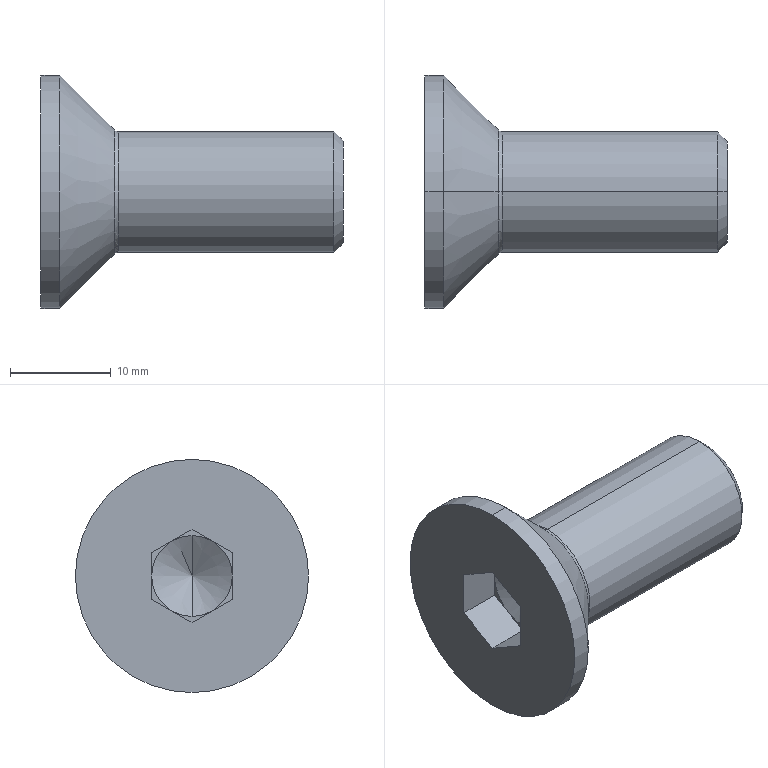Part | STEP file | 1 solid | 26 faces | box 30 x 23.12 x 23.12 mm | volume 4440 mm3 | plane 14 | cone 6 | cylinder 4 | torus 2 | commonest cylinder face diameters 12 x2 23.12 x2